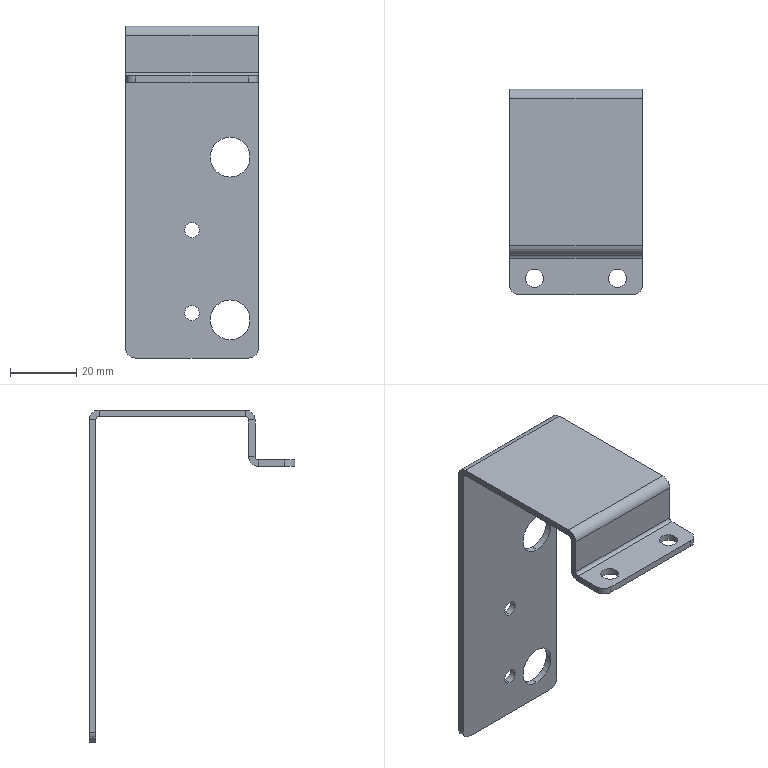Part | SolidWorks | features HoleWzd 3, Fillet 1, FlatPattern 1, SMBaseFlange 1, SheetMetal 1 | 1 solid | 46 faces | box 40 x 62 x 100 mm | volume 13167 mm3 | plane 24 | cylinder 22 | commonest cylinder face diameters 6 x7 4.5 x4 5.5 x4 12 x4 2 x3
STEP:
#1=CARTESIAN_POINT('',(31.5,50.,-94.5));
#2=VERTEX_POINT('',#1);
#3=CARTESIAN_POINT('',(31.5,50.,-82.5));
#4=VERTEX_POINT('',#3);
#5=CARTESIAN_POINT('',(31.5,50.,-88.5));
#6=DIRECTION('',(0.,1.,0.));
#7=DIRECTION('',(0.,0.,1.));
#8=AXIS2_PLACEMENT_3D('',#5,#6,#7);
#9=CIRCLE('',#8,6.);
#10=EDGE_CURVE('',#2,#4,#9,.T.);
#11=ORIENTED_EDGE('',*,*,#10,.T.);
#12=CARTESIAN_POINT('',(31.5,48.,-82.5));
#13=VERTEX_POINT('',#12);
#14=CARTESIAN_POINT('',(31.5,48.,-82.5));
#15=DIRECTION('',(0.,-1.,0.));
#16=VECTOR('',#15,1000.);
#17=LINE('',#14,#16);
#18=EDGE_CURVE('',#4,#13,#17,.T.);
#19=ORIENTED_EDGE('',*,*,#18,.T.);
#20=CARTESIAN_POINT('',(31.5,48.,-94.5));
#21=VERTEX_POINT('',#20);
#22=CARTESIAN_POINT('',(31.5,48.,-88.5));
#23=DIRECTION('',(0.,-1.,0.));
#24=DIRECTION('',(0.,0.,-1.));
#25=AXIS2_PLACEMENT_3D('',#22,#23,#24);
#26=CIRCLE('',#25,6.);
#27=EDGE_CURVE('',#13,#21,#26,.T.);
#28=ORIENTED_EDGE('',*,*,#27,.T.);
#29=CARTESIAN_POINT('',(31.5,48.,-94.5));
#30=DIRECTION('',(0.,-1.,0.));
#31=VECTOR('',#30,1000.);
#32=LINE('',#29,#31);
#33=EDGE_CURVE('',#2,#21,#32,.T.);
#34=ORIENTED_EDGE('',*,*,#33,.F.);
#35=EDGE_LOOP('',(#11,#19,#28,#34));
#36=FACE_OUTER_BOUND('',#35,.T.);
#37=CARTESIAN_POINT('',(31.5,48.,-88.5));
#38=DIRECTION('',(0.,-1.,0.));
#39=DIRECTION('',(0.,0.,-1.));
#40=AXIS2_PLACEMENT_3D('',#37,#38,#39);
#41=CYLINDRICAL_SURFACE('',#40,6.);
#42=ADVANCED_FACE('',(#36),#41,.F.);
#43=CARTESIAN_POINT('',(31.5,50.,-45.5));
#44=VERTEX_POINT('',#43);
#45=CARTESIAN_POINT('',(31.5,50.,-33.5));
#46=VERTEX_POINT('',#45);
#47=CARTESIAN_POINT('',(31.5,50.,-39.5));
#48=DIRECTION('',(0.,1.,0.));
#49=DIRECTION('',(0.,0.,1.));
#50=AXIS2_PLACEMENT_3D('',#47,#48,#49);
#51=CIRCLE('',#50,6.);
#52=EDGE_CURVE('',#44,#46,#51,.T.);
#53=ORIENTED_EDGE('',*,*,#52,.T.);
#54=CARTESIAN_POINT('',(31.5,48.,-33.5));
#55=VERTEX_POINT('',#54);
#56=CARTESIAN_POINT('',(31.5,48.,-33.5));
#57=DIRECTION('',(0.,-1.,0.));
#58=VECTOR('',#57,1000.);
#59=LINE('',#56,#58);
#60=EDGE_CURVE('',#46,#55,#59,.T.);
#61=ORIENTED_EDGE('',*,*,#60,.T.);
#62=CARTESIAN_POINT('',(31.5,48.,-45.5));
#63=VERTEX_POINT('',#62);
#64=CARTESIAN_POINT('',(31.5,48.,-39.5));
#65=DIRECTION('',(0.,-1.,0.));
#66=DIRECTION('',(0.,0.,-1.));
#67=AXIS2_PLACEMENT_3D('',#64,#65,#66);
#68=CIRCLE('',#67,6.);
#69=EDGE_CURVE('',#55,#63,#68,.T.);
#70=ORIENTED_EDGE('',*,*,#69,.T.);
#71=CARTESIAN_POINT('',(31.5,48.,-45.5));
#72=DIRECTION('',(0.,-1.,0.));
#73=VECTOR('',#72,1000.);
#74=LINE('',#71,#73);
#75=EDGE_CURVE('',#44,#63,#74,.T.);
#76=ORIENTED_EDGE('',*,*,#75,.F.);
#77=EDGE_LOOP('',(#53,#61,#70,#76));
#78=FACE_OUTER_BOUND('',#77,.T.);
#79=CARTESIAN_POINT('',(31.5,48.,-39.5));
#80=DIRECTION('',(0.,-1.,0.));
#81=DIRECTION('',(0.,0.,-1.));
#82=AXIS2_PLACEMENT_3D('',#79,#80,#81);
#83=CYLINDRICAL_SURFACE('',#82,6.);
#84=ADVANCED_FACE('',(#78),#83,.F.);
#85=CARTESIAN_POINT('',(20.,48.,-88.75));
#86=VERTEX_POINT('',#85);
#87=CARTESIAN_POINT('',(20.,48.,-84.25));
#88=VERTEX_POINT('',#87);
#89=CARTESIAN_POINT('',(20.,48.,-86.5));
#90=DIRECTION('',(0.,1.,0.));
#91=DIRECTION('',(0.,0.,1.));
#92=AXIS2_PLACEMENT_3D('',#89,#90,#91);
#93=CIRCLE('',#92,2.25);
#94=EDGE_CURVE('',#86,#88,#93,.T.);
#95=ORIENTED_EDGE('',*,*,#94,.F.);
#96=CARTESIAN_POINT('',(20.,50.,-88.75));
#97=VERTEX_POINT('',#96);
#98=CARTESIAN_POINT('',(20.,50.,-88.75));
#99=DIRECTION('',(0.,1.,0.));
#100=VECTOR('',#99,1000.);
#101=LINE('',#98,#100);
#102=EDGE_CURVE('',#86,#97,#101,.T.);
#103=ORIENTED_EDGE('',*,*,#102,.T.);
#104=CARTESIAN_POINT('',(20.,50.,-84.25));
#105=VERTEX_POINT('',#104);
#106=CARTESIAN_POINT('',(20.,50.,-86.5));
#107=DIRECTION('',(0.,1.,0.));
#108=DIRECTION('',(0.,0.,1.));
#109=AXIS2_PLACEMENT_3D('',#106,#107,#108);
#110=CIRCLE('',#109,2.25);
#111=EDGE_CURVE('',#97,#105,#110,.T.);
#112=ORIENTED_EDGE('',*,*,#111,.T.);
#113=CARTESIAN_POINT('',(20.,50.,-84.25));
#114=DIRECTION('',(0.,1.,0.));
#115=VECTOR('',#114,1000.);
#116=LINE('',#113,#115);
#117=EDGE_CURVE('',#88,#105,#116,.T.);
#118=ORIENTED_EDGE('',*,*,#117,.F.);
#119=EDGE_LOOP('',(#95,#103,#112,#118));
#120=FACE_OUTER_BOUND('',#119,.T.);
#121=CARTESIAN_POINT('',(20.,50.,-86.5));
#122=DIRECTION('',(0.,1.,0.));
#123=DIRECTION('',(0.,0.,1.));
#124=AXIS2_PLACEMENT_3D('',#121,#122,#123);
#125=CYLINDRICAL_SURFACE('',#124,2.25);
#126=ADVANCED_FACE('',(#120),#125,.F.);
#127=CARTESIAN_POINT('',(20.,48.,-63.75));
#128=VERTEX_POINT('',#127);
#129=CARTESIAN_POINT('',(20.,48.,-59.25));
#130=VERTEX_POINT('',#129);
#131=CARTESIAN_POINT('',(20.,48.,-61.5));
#132=DIRECTION('',(0.,1.,0.));
#133=DIRECTION('',(0.,0.,1.));
#134=AXIS2_PLACEMENT_3D('',#131,#132,#133);
#135=CIRCLE('',#134,2.25);
#136=EDGE_CURVE('',#128,#130,#135,.T.);
#137=ORIENTED_EDGE('',*,*,#136,.F.);
#138=CARTESIAN_POINT('',(20.,50.,-63.75));
#139=VERTEX_POINT('',#138);
#140=CARTESIAN_POINT('',(20.,50.,-63.75));
#141=DIRECTION('',(0.,1.,0.));
#142=VECTOR('',#141,1000.);
#143=LINE('',#140,#142);
#144=EDGE_CURVE('',#128,#139,#143,.T.);
#145=ORIENTED_EDGE('',*,*,#144,.T.);
#146=CARTESIAN_POINT('',(20.,50.,-59.25));
#147=VERTEX_POINT('',#146);
#148=CARTESIAN_POINT('',(20.,50.,-61.5));
#149=DIRECTION('',(0.,1.,0.));
#150=DIRECTION('',(0.,0.,1.));
#151=AXIS2_PLACEMENT_3D('',#148,#149,#150);
#152=CIRCLE('',#151,2.25);
#153=EDGE_CURVE('',#139,#147,#152,.T.);
#154=ORIENTED_EDGE('',*,*,#153,.T.);
#155=CARTESIAN_POINT('',(20.,50.,-59.25));
#156=DIRECTION('',(0.,1.,0.));
#157=VECTOR('',#156,1000.);
#158=LINE('',#155,#157);
#159=EDGE_CURVE('',#130,#147,#158,.T.);
#160=ORIENTED_EDGE('',*,*,#159,.F.);
#161=EDGE_LOOP('',(#137,#145,#154,#160));
#162=FACE_OUTER_BOUND('',#161,.T.);
#163=CARTESIAN_POINT('',(20.,50.,-61.5));
#164=DIRECTION('',(0.,1.,0.));
#165=DIRECTION('',(0.,0.,1.));
#166=AXIS2_PLACEMENT_3D('',#163,#164,#165);
#167=CYLINDRICAL_SURFACE('',#166,2.25);
#168=ADVANCED_FACE('',(#162),#167,.F.);
#169=CARTESIAN_POINT('',(4.75,-7.,-17.));
#170=VERTEX_POINT('',#169);
#171=CARTESIAN_POINT('',(10.25,-7.,-17.));
#172=VERTEX_POINT('',#171);
#173=CARTESIAN_POINT('',(7.5,-7.,-17.));
#174=DIRECTION('',(0.,0.,1.));
#175=DIRECTION('',(0.,-1.,0.));
#176=AXIS2_PLACEMENT_3D('',#173,#174,#175);
#177=CIRCLE('',#176,2.75);
#178=EDGE_CURVE('',#170,#172,#177,.T.);
#179=ORIENTED_EDGE('',*,*,#178,.F.);
#180=CARTESIAN_POINT('',(4.75,-7.,-15.));
#181=VERTEX_POINT('',#180);
#182=CARTESIAN_POINT('',(4.75,-7.,-15.));
#183=DIRECTION('',(0.,0.,1.));
#184=VECTOR('',#183,1000.);
#185=LINE('',#182,#184);
#186=EDGE_CURVE('',#170,#181,#185,.T.);
#187=ORIENTED_EDGE('',*,*,#186,.T.);
#188=CARTESIAN_POINT('',(10.25,-7.,-15.));
#189=VERTEX_POINT('',#188);
#190=CARTESIAN_POINT('',(7.5,-7.,-15.));
#191=DIRECTION('',(0.,0.,1.));
#192=DIRECTION('',(1.,0.,0.));
#193=AXIS2_PLACEMENT_3D('',#190,#191,#192);
#194=CIRCLE('',#193,2.75);
#195=EDGE_CURVE('',#181,#189,#194,.T.);
#196=ORIENTED_EDGE('',*,*,#195,.T.);
#197=CARTESIAN_POINT('',(10.25,-7.,-15.));
#198=DIRECTION('',(0.,0.,1.));
#199=VECTOR('',#198,1000.);
#200=LINE('',#197,#199);
#201=EDGE_CURVE('',#172,#189,#200,.T.);
#202=ORIENTED_EDGE('',*,*,#201,.F.);
#203=EDGE_LOOP('',(#179,#187,#196,#202));
#204=FACE_OUTER_BOUND('',#203,.T.);
#205=CARTESIAN_POINT('',(7.5,-7.,-15.));
#206=DIRECTION('',(0.,0.,1.));
#207=DIRECTION('',(1.,0.,0.));
#208=AXIS2_PLACEMENT_3D('',#205,#206,#207);
#209=CYLINDRICAL_SURFACE('',#208,2.75);
#210=ADVANCED_FACE('',(#204),#209,.F.);
#211=CARTESIAN_POINT('',(29.75,-7.,-17.));
#212=VERTEX_POINT('',#211);
#213=CARTESIAN_POINT('',(35.25,-7.,-17.));
#214=VERTEX_POINT('',#213);
#215=CARTESIAN_POINT('',(32.5,-7.,-17.));
#216=DIRECTION('',(0.,0.,1.));
#217=DIRECTION('',(0.,-1.,0.));
#218=AXIS2_PLACEMENT_3D('',#215,#216,#217);
#219=CIRCLE('',#218,2.75);
#220=EDGE_CURVE('',#212,#214,#219,.T.);
#221=ORIENTED_EDGE('',*,*,#220,.F.);
#222=CARTESIAN_POINT('',(29.75,-7.,-15.));
#223=VERTEX_POINT('',#222);
#224=CARTESIAN_POINT('',(29.75,-7.,-15.));
#225=DIRECTION('',(0.,0.,1.));
#226=VECTOR('',#225,1000.);
#227=LINE('',#224,#226);
#228=EDGE_CURVE('',#212,#223,#227,.T.);
#229=ORIENTED_EDGE('',*,*,#228,.T.);
#230=CARTESIAN_POINT('',(35.25,-7.,-15.));
#231=VERTEX_POINT('',#230);
#232=CARTESIAN_POINT('',(32.5,-7.,-15.));
#233=DIRECTION('',(0.,0.,1.));
#234=DIRECTION('',(1.,0.,0.));
#235=AXIS2_PLACEMENT_3D('',#232,#233,#234);
#236=CIRCLE('',#235,2.75);
#237=EDGE_CURVE('',#223,#231,#236,.T.);
#238=ORIENTED_EDGE('',*,*,#237,.T.);
#239=CARTESIAN_POINT('',(35.25,-7.,-15.));
#240=DIRECTION('',(0.,0.,1.));
#241=VECTOR('',#240,1000.);
#242=LINE('',#239,#241);
#243=EDGE_CURVE('',#214,#231,#242,.T.);
#244=ORIENTED_EDGE('',*,*,#243,.F.);
#245=EDGE_LOOP('',(#221,#229,#238,#244));
#246=FACE_OUTER_BOUND('',#245,.T.);
#247=CARTESIAN_POINT('',(32.5,-7.,-15.));
#248=DIRECTION('',(0.,0.,1.));
#249=DIRECTION('',(1.,0.,0.));
#250=AXIS2_PLACEMENT_3D('',#247,#248,#249);
#251=CYLINDRICAL_SURFACE('',#250,2.75);
#252=ADVANCED_FACE('',(#246),#251,.F.);
#253=CARTESIAN_POINT('',(40.,0.,-14.));
#254=VERTEX_POINT('',#253);
#255=CARTESIAN_POINT('',(40.,2.,-14.));
#256=VERTEX_POINT('',#255);
#257=CARTESIAN_POINT('',(40.,0.,-14.));
#258=DIRECTION('',(0.,1.,0.));
#259=VECTOR('',#258,1000.);
#260=LINE('',#257,#259);
#261=EDGE_CURVE('',#254,#256,#260,.T.);
#262=ORIENTED_EDGE('',*,*,#261,.F.);
#263=CARTESIAN_POINT('',(40.,-1.,-15.));
#264=VERTEX_POINT('',#263);
#265=CARTESIAN_POINT('',(40.,-1.,-14.));
#266=DIRECTION('',(1.,0.,0.));
#267=DIRECTION('',(0.,0.,1.));
#268=AXIS2_PLACEMENT_3D('',#265,#266,#267);
#269=CIRCLE('',#268,1.);
#270=EDGE_CURVE('',#264,#254,#269,.T.);
#271=ORIENTED_EDGE('',*,*,#270,.F.);
#272=CARTESIAN_POINT('',(40.,-1.,-17.));
#273=VERTEX_POINT('',#272);
#274=CARTESIAN_POINT('',(40.,-1.,-17.));
#275=DIRECTION('',(0.,0.,1.));
#276=VECTOR('',#275,1000.);
#277=LINE('',#274,#276);
#278=EDGE_CURVE('',#273,#264,#277,.T.);
#279=ORIENTED_EDGE('',*,*,#278,.F.);
#280=CARTESIAN_POINT('',(40.,-1.,-14.));
#281=DIRECTION('',(1.,0.,0.));
#282=DIRECTION('',(0.,0.,-1.));
#283=AXIS2_PLACEMENT_3D('',#280,#281,#282);
#284=CIRCLE('',#283,3.);
#285=EDGE_CURVE('',#273,#256,#284,.T.);
#286=ORIENTED_EDGE('',*,*,#285,.T.);
#287=EDGE_LOOP('',(#262,#271,#279,#286));
#288=FACE_OUTER_BOUND('',#287,.T.);
#289=CARTESIAN_POINT('',(40.,0.,-14.));
#290=DIRECTION('',(1.,0.,0.));
#291=DIRECTION('',(0.,0.,-1.));
#292=AXIS2_PLACEMENT_3D('',#289,#290,#291);
#293=PLANE('',#292);
#294=ADVANCED_FACE('',(#288),#293,.T.);
#295=CARTESIAN_POINT('',(40.,0.,-3.));
#296=VERTEX_POINT('',#295);
#297=CARTESIAN_POINT('',(40.,0.,0.));
#298=DIRECTION('',(0.,0.,1.));
#299=VECTOR('',#298,1000.);
#300=LINE('',#297,#299);
#301=EDGE_CURVE('',#254,#296,#300,.T.);
#302=ORIENTED_EDGE('',*,*,#301,.F.);
#303=ORIENTED_EDGE('',*,*,#261,.T.);
#304=CARTESIAN_POINT('',(40.,2.,-3.));
#305=VERTEX_POINT('',#304);
#306=CARTESIAN_POINT('',(40.,2.,0.));
#307=DIRECTION('',(0.,0.,1.));
#308=VECTOR('',#307,1000.);
#309=LINE('',#306,#308);
#310=EDGE_CURVE('',#256,#305,#309,.T.);
#311=ORIENTED_EDGE('',*,*,#310,.T.);
#312=CARTESIAN_POINT('',(40.,2.,-3.));
#313=DIRECTION('',(0.,-1.,0.));
#314=VECTOR('',#313,1000.);
#315=LINE('',#312,#314);
#316=EDGE_CURVE('',#305,#296,#315,.T.);
#317=ORIENTED_EDGE('',*,*,#316,.T.);
#318=EDGE_LOOP('',(#302,#303,#311,#317));
#319=FACE_OUTER_BOUND('',#318,.T.);
#320=CARTESIAN_POINT('',(40.,-1.,-17.));
#321=DIRECTION('',(1.,0.,0.));
#322=DIRECTION('',(0.,0.,-1.));
#323=AXIS2_PLACEMENT_3D('',#320,#321,#322);
#324=PLANE('',#323);
#325=ADVANCED_FACE('',(#319),#324,.T.);
#326=CARTESIAN_POINT('',(0.,-1.,-15.));
#327=VERTEX_POINT('',#326);
#328=CARTESIAN_POINT('',(0.,-1.,-17.));
#329=VERTEX_POINT('',#328);
#330=CARTESIAN_POINT('',(0.,-1.,-15.));
#331=DIRECTION('',(0.,0.,-1.));
#332=VECTOR('',#331,1000.);
#333=LINE('',#330,#332);
#334=EDGE_CURVE('',#327,#329,#333,.T.);
#335=ORIENTED_EDGE('',*,*,#334,.F.);
#336=CARTESIAN_POINT('',(0.,0.,-14.));
#337=VERTEX_POINT('',#336);
#338=CARTESIAN_POINT('',(0.,-1.,-14.));
#339=DIRECTION('',(1.,0.,0.));
#340=DIRECTION('',(0.,0.,1.));
#341=AXIS2_PLACEMENT_3D('',#338,#339,#340);
#342=CIRCLE('',#341,1.);
#343=EDGE_CURVE('',#327,#337,#342,.T.);
#344=ORIENTED_EDGE('',*,*,#343,.T.);
#345=CARTESIAN_POINT('',(0.,2.,-14.));
#346=VERTEX_POINT('',#345);
#347=CARTESIAN_POINT('',(0.,2.,-14.));
#348=DIRECTION('',(0.,-1.,0.));
#349=VECTOR('',#348,1000.);
#350=LINE('',#347,#349);
#351=EDGE_CURVE('',#346,#337,#350,.T.);
#352=ORIENTED_EDGE('',*,*,#351,.F.);
#353=CARTESIAN_POINT('',(0.,-1.,-14.));
#354=DIRECTION('',(1.,0.,0.));
#355=DIRECTION('',(0.,0.,-1.));
#356=AXIS2_PLACEMENT_3D('',#353,#354,#355);
#357=CIRCLE('',#356,3.);
#358=EDGE_CURVE('',#329,#346,#357,.T.);
#359=ORIENTED_EDGE('',*,*,#358,.F.);
#360=EDGE_LOOP('',(#335,#344,#352,#359));
#361=FACE_OUTER_BOUND('',#360,.T.);
#362=CARTESIAN_POINT('',(0.,-1.,-15.));
#363=DIRECTION('',(-1.,0.,0.));
#364=DIRECTION('',(0.,0.,1.));
#365=AXIS2_PLACEMENT_3D('',#362,#363,#364);
#366=PLANE('',#365);
#367=ADVANCED_FACE('',(#361),#366,.T.);
#368=CARTESIAN_POINT('',(0.,-9.,-17.));
#369=VERTEX_POINT('',#368);
#370=CARTESIAN_POINT('',(0.,0.,-17.));
#371=DIRECTION('',(0.,1.,0.));
#372=VECTOR('',#371,1000.);
#373=LINE('',#370,#372);
#374=EDGE_CURVE('',#369,#329,#373,.T.);
#375=ORIENTED_EDGE('',*,*,#374,.F.);
#376=CARTESIAN_POINT('',(0.,-9.,-15.));
#377=VERTEX_POINT('',#376);
#378=CARTESIAN_POINT('',(0.,-9.,-14.));
#379=DIRECTION('',(0.,0.,1.));
#380=VECTOR('',#379,1000.);
#381=LINE('',#378,#380);
#382=EDGE_CURVE('',#369,#377,#381,.T.);
#383=ORIENTED_EDGE('',*,*,#382,.T.);
#384=CARTESIAN_POINT('',(0.,0.,-15.));
#385=DIRECTION('',(0.,1.,0.));
#386=VECTOR('',#385,1000.);
#387=LINE('',#384,#386);
#388=EDGE_CURVE('',#377,#327,#387,.T.);
#389=ORIENTED_EDGE('',*,*,#388,.T.);
#390=ORIENTED_EDGE('',*,*,#334,.T.);
#391=EDGE_LOOP('',(#375,#383,#389,#390));
#392=FACE_OUTER_BOUND('',#391,.T.);
#393=CARTESIAN_POINT('',(0.,2.,-14.));
#394=DIRECTION('',(-1.,0.,0.));
#395=DIRECTION('',(0.,0.,1.));
#396=AXIS2_PLACEMENT_3D('',#393,#394,#395);
#397=PLANE('',#396);
#398=ADVANCED_FACE('',(#392),#397,.T.);
#399=CARTESIAN_POINT('',(40.,3.,0.));
#400=VERTEX_POINT('',#399);
#401=CARTESIAN_POINT('',(40.,3.,-2.));
#402=VERTEX_POINT('',#401);
#403=CARTESIAN_POINT('',(40.,3.,0.));
#404=DIRECTION('',(0.,0.,-1.));
#405=VECTOR('',#404,1000.);
#406=LINE('',#403,#405);
#407=EDGE_CURVE('',#400,#402,#406,.T.);
#408=ORIENTED_EDGE('',*,*,#407,.F.);
#409=CARTESIAN_POINT('',(40.,3.,-3.));
#410=DIRECTION('',(-1.,0.,0.));
#411=DIRECTION('',(0.,0.,-1.));
#412=AXIS2_PLACEMENT_3D('',#409,#410,#411);
#413=CIRCLE('',#412,3.);
#414=EDGE_CURVE('',#296,#400,#413,.T.);
#415=ORIENTED_EDGE('',*,*,#414,.F.);
#416=ORIENTED_EDGE('',*,*,#316,.F.);
#417=CARTESIAN_POINT('',(40.,3.,-3.));
#418=DIRECTION('',(-1.,0.,0.));
#419=DIRECTION('',(0.,0.,-1.));
#420=AXIS2_PLACEMENT_3D('',#417,#418,#419);
#421=CIRCLE('',#420,1.);
#422=EDGE_CURVE('',#305,#402,#421,.T.);
#423=ORIENTED_EDGE('',*,*,#422,.T.);
#424=EDGE_LOOP('',(#408,#415,#416,#423));
#425=FACE_OUTER_BOUND('',#424,.T.);
#426=CARTESIAN_POINT('',(40.,3.,0.));
#427=DIRECTION('',(1.,0.,0.));
#428=DIRECTION('',(0.,0.,-1.));
#429=AXIS2_PLACEMENT_3D('',#426,#427,#428);
#430=PLANE('',#429);
#431=ADVANCED_FACE('',(#425),#430,.T.);
#432=CARTESIAN_POINT('',(40.,47.,0.));
#433=VERTEX_POINT('',#432);
#434=CARTESIAN_POINT('',(40.,0.,0.));
#435=DIRECTION('',(0.,1.,0.));
#436=VECTOR('',#435,1000.);
#437=LINE('',#434,#436);
#438=EDGE_CURVE('',#400,#433,#437,.T.);
#439=ORIENTED_EDGE('',*,*,#438,.F.);
#440=ORIENTED_EDGE('',*,*,#407,.T.);
#441=CARTESIAN_POINT('',(40.,47.,-2.));
#442=VERTEX_POINT('',#441);
#443=CARTESIAN_POINT('',(40.,0.,-2.));
#444=DIRECTION('',(0.,1.,0.));
#445=VECTOR('',#444,1000.);
#446=LINE('',#443,#445);
#447=EDGE_CURVE('',#402,#442,#446,.T.);
#448=ORIENTED_EDGE('',*,*,#447,.T.);
#449=CARTESIAN_POINT('',(40.,47.,-2.));
#450=DIRECTION('',(0.,0.,1.));
#451=VECTOR('',#450,1000.);
#452=LINE('',#449,#451);
#453=EDGE_CURVE('',#442,#433,#452,.T.);
#454=ORIENTED_EDGE('',*,*,#453,.T.);
#455=EDGE_LOOP('',(#439,#440,#448,#454));
#456=FACE_OUTER_BOUND('',#455,.T.);
#457=CARTESIAN_POINT('',(40.,2.,-3.));
#458=DIRECTION('',(1.,0.,0.));
#459=DIRECTION('',(0.,0.,-1.));
#460=AXIS2_PLACEMENT_3D('',#457,#458,#459);
#461=PLANE('',#460);
#462=ADVANCED_FACE('',(#456),#461,.T.);
#463=CARTESIAN_POINT('',(0.,0.,-3.));
#464=VERTEX_POINT('',#463);
#465=CARTESIAN_POINT('',(0.,2.,-3.));
#466=VERTEX_POINT('',#465);
#467=CARTESIAN_POINT('',(0.,0.,-3.));
#468=DIRECTION('',(0.,1.,0.));
#469=VECTOR('',#468,1000.);
#470=LINE('',#467,#469);
#471=EDGE_CURVE('',#464,#466,#470,.T.);
#472=ORIENTED_EDGE('',*,*,#471,.F.);
#473=CARTESIAN_POINT('',(0.,3.,0.));
#474=VERTEX_POINT('',#473);
#475=CARTESIAN_POINT('',(0.,3.,-3.));
#476=DIRECTION('',(-1.,0.,0.));
#477=DIRECTION('',(0.,0.,-1.));
#478=AXIS2_PLACEMENT_3D('',#475,#476,#477);
#479=CIRCLE('',#478,3.);
#480=EDGE_CURVE('',#464,#474,#479,.T.);
#481=ORIENTED_EDGE('',*,*,#480,.T.);
#482=CARTESIAN_POINT('',(0.,3.,-2.));
#483=VERTEX_POINT('',#482);
#484=CARTESIAN_POINT('',(0.,3.,-2.));
#485=DIRECTION('',(0.,0.,1.));
#486=VECTOR('',#485,1000.);
#487=LINE('',#484,#486);
#488=EDGE_CURVE('',#483,#474,#487,.T.);
#489=ORIENTED_EDGE('',*,*,#488,.F.);
#490=CARTESIAN_POINT('',(0.,3.,-3.));
#491=DIRECTION('',(-1.,0.,0.));
#492=DIRECTION('',(0.,0.,-1.));
#493=AXIS2_PLACEMENT_3D('',#490,#491,#492);
#494=CIRCLE('',#493,1.);
#495=EDGE_CURVE('',#466,#483,#494,.T.);
#496=ORIENTED_EDGE('',*,*,#495,.F.);
#497=EDGE_LOOP('',(#472,#481,#489,#496));
#498=FACE_OUTER_BOUND('',#497,.T.);
#499=CARTESIAN_POINT('',(0.,0.,-3.));
#500=DIRECTION('',(-1.,0.,0.));
#501=DIRECTION('',(0.,0.,1.));
#502=AXIS2_PLACEMENT_3D('',#499,#500,#501);
#503=PLANE('',#502);
#504=ADVANCED_FACE('',(#498),#503,.T.);
#505=CARTESIAN_POINT('',(0.,0.,0.));
#506=DIRECTION('',(0.,0.,1.));
#507=VECTOR('',#506,1000.);
#508=LINE('',#505,#507);
#509=EDGE_CURVE('',#337,#464,#508,.T.);
#510=ORIENTED_EDGE('',*,*,#509,.T.);
#511=ORIENTED_EDGE('',*,*,#471,.T.);
#512=CARTESIAN_POINT('',(0.,2.,0.));
#513=DIRECTION('',(0.,0.,1.));
#514=VECTOR('',#513,1000.);
#515=LINE('',#512,#514);
#516=EDGE_CURVE('',#346,#466,#515,.T.);
#517=ORIENTED_EDGE('',*,*,#516,.F.);
#518=ORIENTED_EDGE('',*,*,#351,.T.);
#519=EDGE_LOOP('',(#510,#511,#517,#518));
#520=FACE_OUTER_BOUND('',#519,.T.);
#521=CARTESIAN_POINT('',(0.,3.,-2.));
#522=DIRECTION('',(-1.,0.,0.));
#523=DIRECTION('',(0.,0.,1.));
#524=AXIS2_PLACEMENT_3D('',#521,#522,#523);
#525=PLANE('',#524);
#526=ADVANCED_FACE('',(#520),#525,.T.);
#527=CARTESIAN_POINT('',(40.,50.,-3.));
#528=VERTEX_POINT('',#527);
#529=CARTESIAN_POINT('',(40.,48.,-3.));
#530=VERTEX_POINT('',#529);
#531=CARTESIAN_POINT('',(40.,50.,-3.));
#532=DIRECTION('',(0.,-1.,0.));
#533=VECTOR('',#532,1000.);
#534=LINE('',#531,#533);
#535=EDGE_CURVE('',#528,#530,#534,.T.);
#536=ORIENTED_EDGE('',*,*,#535,.F.);
#537=CARTESIAN_POINT('',(40.,47.,-3.));
#538=DIRECTION('',(-1.,0.,0.));
#539=DIRECTION('',(0.,0.,-1.));
#540=AXIS2_PLACEMENT_3D('',#537,#538,#539);
#541=CIRCLE('',#540,3.);
#542=EDGE_CURVE('',#433,#528,#541,.T.);
#543=ORIENTED_EDGE('',*,*,#542,.F.);
#544=ORIENTED_EDGE('',*,*,#453,.F.);
#545=CARTESIAN_POINT('',(40.,47.,-3.));
#546=DIRECTION('',(-1.,0.,0.));
#547=DIRECTION('',(0.,0.,-1.));
#548=AXIS2_PLACEMENT_3D('',#545,#546,#547);
#549=CIRCLE('',#548,1.);
#550=EDGE_CURVE('',#442,#530,#549,.T.);
#551=ORIENTED_EDGE('',*,*,#550,.T.);
#552=EDGE_LOOP('',(#536,#543,#544,#551));
#553=FACE_OUTER_BOUND('',#552,.T.);
#554=CARTESIAN_POINT('',(40.,50.,-3.));
#555=DIRECTION('',(1.,0.,0.));
#556=DIRECTION('',(0.,0.,-1.));
#557=AXIS2_PLACEMENT_3D('',#554,#555,#556);
#558=PLANE('',#557);
#559=ADVANCED_FACE('',(#553),#558,.T.);
#560=CARTESIAN_POINT('',(40.,48.,-97.));
#561=VERTEX_POINT('',#560);
#562=CARTESIAN_POINT('',(40.,48.,0.));
#563=DIRECTION('',(0.,0.,-1.));
#564=VECTOR('',#563,1000.);
#565=LINE('',#562,#564);
#566=EDGE_CURVE('',#530,#561,#565,.T.);
#567=ORIENTED_EDGE('',*,*,#566,.T.);
#568=CARTESIAN_POINT('',(40.,50.,-97.));
#569=VERTEX_POINT('',#568);
#570=CARTESIAN_POINT('',(40.,47.,-97.));
#571=DIRECTION('',(0.,1.,0.));
#572=VECTOR('',#571,1000.);
#573=LINE('',#570,#572);
#574=EDGE_CURVE('',#561,#569,#573,.T.);
#575=ORIENTED_EDGE('',*,*,#574,.T.);
#576=CARTESIAN_POINT('',(40.,50.,0.));
#577=DIRECTION('',(0.,0.,-1.));
#578=VECTOR('',#577,1000.);
#579=LINE('',#576,#578);
#580=EDGE_CURVE('',#528,#569,#579,.T.);
#581=ORIENTED_EDGE('',*,*,#580,.F.);
#582=ORIENTED_EDGE('',*,*,#535,.T.);
#583=EDGE_LOOP('',(#567,#575,#581,#582));
#584=FACE_OUTER_BOUND('',#583,.T.);
#585=CARTESIAN_POINT('',(40.,47.,-2.));
#586=DIRECTION('',(1.,0.,0.));
#587=DIRECTION('',(0.,0.,-1.));
#588=AXIS2_PLACEMENT_3D('',#585,#586,#587);
#589=PLANE('',#588);
#590=ADVANCED_FACE('',(#584),#589,.T.);
#591=CARTESIAN_POINT('',(0.,47.,0.));
#592=VERTEX_POINT('',#591);
#593=CARTESIAN_POINT('',(0.,47.,-2.));
#594=VERTEX_POINT('',#593);
#595=CARTESIAN_POINT('',(0.,47.,0.));
#596=DIRECTION('',(0.,0.,-1.));
#597=VECTOR('',#596,1000.);
#598=LINE('',#595,#597);
#599=EDGE_CURVE('',#592,#594,#598,.T.);
#600=ORIENTED_EDGE('',*,*,#599,.F.);
#601=CARTESIAN_POINT('',(0.,50.,-3.));
#602=VERTEX_POINT('',#601);
#603=CARTESIAN_POINT('',(0.,47.,-3.));
#604=DIRECTION('',(-1.,0.,0.));
#605=DIRECTION('',(0.,0.,-1.));
#606=AXIS2_PLACEMENT_3D('',#603,#604,#605);
#607=CIRCLE('',#606,3.);
#608=EDGE_CURVE('',#592,#602,#607,.T.);
#609=ORIENTED_EDGE('',*,*,#608,.T.);
#610=CARTESIAN_POINT('',(0.,48.,-3.));
#611=VERTEX_POINT('',#610);
#612=CARTESIAN_POINT('',(0.,48.,-3.));
#613=DIRECTION('',(0.,1.,0.));
#614=VECTOR('',#613,1000.);
#615=LINE('',#612,#614);
#616=EDGE_CURVE('',#611,#602,#615,.T.);
#617=ORIENTED_EDGE('',*,*,#616,.F.);
#618=CARTESIAN_POINT('',(0.,47.,-3.));
#619=DIRECTION('',(-1.,0.,0.));
#620=DIRECTION('',(0.,0.,-1.));
#621=AXIS2_PLACEMENT_3D('',#618,#619,#620);
#622=CIRCLE('',#621,1.);
#623=EDGE_CURVE('',#594,#611,#622,.T.);
#624=ORIENTED_EDGE('',*,*,#623,.F.);
#625=EDGE_LOOP('',(#600,#609,#617,#624));
#626=FACE_OUTER_BOUND('',#625,.T.);
#627=CARTESIAN_POINT('',(0.,47.,0.));
#628=DIRECTION('',(-1.,0.,0.));
#629=DIRECTION('',(0.,0.,1.));
#630=AXIS2_PLACEMENT_3D('',#627,#628,#629);
#631=PLANE('',#630);
#632=ADVANCED_FACE('',(#626),#631,.T.);
#633=CARTESIAN_POINT('',(0.,0.,0.));
#634=DIRECTION('',(0.,1.,0.));
#635=VECTOR('',#634,1000.);
#636=LINE('',#633,#635);
#637=EDGE_CURVE('',#474,#592,#636,.T.);
#638=ORIENTED_EDGE('',*,*,#637,.T.);
#639=ORIENTED_EDGE('',*,*,#599,.T.);
#640=CARTESIAN_POINT('',(0.,0.,-2.));
#641=DIRECTION('',(0.,1.,0.));
#642=VECTOR('',#641,1000.);
#643=LINE('',#640,#642);
#644=EDGE_CURVE('',#483,#594,#643,.T.);
#645=ORIENTED_EDGE('',*,*,#644,.F.);
#646=ORIENTED_EDGE('',*,*,#488,.T.);
#647=EDGE_LOOP('',(#638,#639,#645,#646));
#648=FACE_OUTER_BOUND('',#647,.T.);
#649=CARTESIAN_POINT('',(0.,48.,-3.));
#650=DIRECTION('',(-1.,0.,0.));
#651=DIRECTION('',(0.,0.,1.));
#652=AXIS2_PLACEMENT_3D('',#649,#650,#651);
#653=PLANE('',#652);
#654=ADVANCED_FACE('',(#648),#653,.T.);
#655=CARTESIAN_POINT('',(31.5,48.,-88.5));
#656=DIRECTION('',(0.,-1.,0.));
#657=DIRECTION('',(0.,0.,-1.));
#658=AXIS2_PLACEMENT_3D('',#655,#656,#657);
#659=CIRCLE('',#658,6.);
#660=EDGE_CURVE('',#21,#13,#659,.T.);
#661=ORIENTED_EDGE('',*,*,#660,.F.);
#662=ORIENTED_EDGE('',*,*,#27,.F.);
#663=EDGE_LOOP('',(#661,#662));
#664=FACE_BOUND('',#663,.T.);
#665=CARTESIAN_POINT('',(31.5,48.,-39.5));
#666=DIRECTION('',(0.,-1.,0.));
#667=DIRECTION('',(0.,0.,-1.));
#668=AXIS2_PLACEMENT_3D('',#665,#666,#667);
#669=CIRCLE('',#668,6.);
#670=EDGE_CURVE('',#63,#55,#669,.T.);
#671=ORIENTED_EDGE('',*,*,#670,.F.);
#672=ORIENTED_EDGE('',*,*,#69,.F.);
#673=EDGE_LOOP('',(#671,#672));
#674=FACE_BOUND('',#673,.T.);
#675=CARTESIAN_POINT('',(20.,48.,-86.5));
#676=DIRECTION('',(0.,1.,0.));
#677=DIRECTION('',(0.,0.,1.));
#678=AXIS2_PLACEMENT_3D('',#675,#676,#677);
#679=CIRCLE('',#678,2.25);
#680=EDGE_CURVE('',#88,#86,#679,.T.);
#681=ORIENTED_EDGE('',*,*,#680,.T.);
#682=ORIENTED_EDGE('',*,*,#94,.T.);
#683=EDGE_LOOP('',(#681,#682));
#684=FACE_BOUND('',#683,.T.);
#685=CARTESIAN_POINT('',(20.,48.,-61.5));
#686=DIRECTION('',(0.,1.,0.));
#687=DIRECTION('',(0.,0.,1.));
#688=AXIS2_PLACEMENT_3D('',#685,#686,#687);
#689=CIRCLE('',#688,2.25);
#690=EDGE_CURVE('',#130,#128,#689,.T.);
#691=ORIENTED_EDGE('',*,*,#690,.T.);
#692=ORIENTED_EDGE('',*,*,#136,.T.);
#693=EDGE_LOOP('',(#691,#692));
#694=FACE_BOUND('',#693,.T.);
#695=CARTESIAN_POINT('',(37.,48.,-100.));
#696=VERTEX_POINT('',#695);
#697=CARTESIAN_POINT('',(3.,48.,-100.));
#698=VERTEX_POINT('',#697);
#699=CARTESIAN_POINT('',(40.,48.,-100.));
#700=DIRECTION('',(-1.,0.,0.));
#701=VECTOR('',#700,1000.);
#702=LINE('',#699,#701);
#703=EDGE_CURVE('',#696,#698,#702,.T.);
#704=ORIENTED_EDGE('',*,*,#703,.F.);
#705=CARTESIAN_POINT('',(37.,48.,-97.));
#706=DIRECTION('',(0.,-1.,0.));
#707=DIRECTION('',(0.,0.,1.));
#708=AXIS2_PLACEMENT_3D('',#705,#706,#707);
#709=CIRCLE('',#708,3.);
#710=EDGE_CURVE('',#696,#561,#709,.T.);
#711=ORIENTED_EDGE('',*,*,#710,.T.);
#712=ORIENTED_EDGE('',*,*,#566,.F.);
#713=CARTESIAN_POINT('',(40.,48.,-3.));
#714=DIRECTION('',(-1.,0.,0.));
#715=VECTOR('',#714,1000.);
#716=LINE('',#713,#715);
#717=EDGE_CURVE('',#530,#611,#716,.T.);
#718=ORIENTED_EDGE('',*,*,#717,.T.);
#719=CARTESIAN_POINT('',(0.,48.,-97.));
#720=VERTEX_POINT('',#719);
#721=CARTESIAN_POINT('',(0.,48.,0.));
#722=DIRECTION('',(0.,0.,-1.));
#723=VECTOR('',#722,1000.);
#724=LINE('',#721,#723);
#725=EDGE_CURVE('',#611,#720,#724,.T.);
#726=ORIENTED_EDGE('',*,*,#725,.T.);
#727=CARTESIAN_POINT('',(3.,48.,-97.));
#728=DIRECTION('',(0.,-1.,0.));
#729=DIRECTION('',(0.,0.,1.));
#730=AXIS2_PLACEMENT_3D('',#727,#728,#729);
#731=CIRCLE('',#730,3.);
#732=EDGE_CURVE('',#720,#698,#731,.T.);
#733=ORIENTED_EDGE('',*,*,#732,.T.);
#734=EDGE_LOOP('',(#704,#711,#712,#718,#726,#733));
#735=FACE_OUTER_BOUND('',#734,.T.);
#736=CARTESIAN_POINT('',(40.,48.,0.));
#737=DIRECTION('',(0.,1.,0.));
#738=DIRECTION('',(0.,0.,1.));
#739=AXIS2_PLACEMENT_3D('',#736,#737,#738);
#740=PLANE('',#739);
#741=ADVANCED_FACE('',(#664,#674,#684,#694,#735),#740,.F.);
#742=CARTESIAN_POINT('',(37.,50.,-100.));
#743=VERTEX_POINT('',#742);
#744=CARTESIAN_POINT('',(3.,50.,-100.));
#745=VERTEX_POINT('',#744);
#746=CARTESIAN_POINT('',(40.,50.,-100.));
#747=DIRECTION('',(-1.,0.,0.));
#748=VECTOR('',#747,1000.);
#749=LINE('',#746,#748);
#750=EDGE_CURVE('',#743,#745,#749,.T.);
#751=ORIENTED_EDGE('',*,*,#750,.F.);
#752=CARTESIAN_POINT('',(37.,50.,-100.));
#753=DIRECTION('',(0.,-1.,0.));
#754=VECTOR('',#753,1000.);
#755=LINE('',#752,#754);
#756=EDGE_CURVE('',#743,#696,#755,.T.);
#757=ORIENTED_EDGE('',*,*,#756,.T.);
#758=ORIENTED_EDGE('',*,*,#703,.T.);
#759=CARTESIAN_POINT('',(3.,50.,-100.));
#760=DIRECTION('',(0.,1.,0.));
#761=VECTOR('',#760,1000.);
#762=LINE('',#759,#761);
#763=EDGE_CURVE('',#698,#745,#762,.T.);
#764=ORIENTED_EDGE('',*,*,#763,.T.);
#765=EDGE_LOOP('',(#751,#757,#758,#764));
#766=FACE_OUTER_BOUND('',#765,.T.);
#767=CARTESIAN_POINT('',(40.,50.,-100.));
#768=DIRECTION('',(0.,0.,-1.));
#769=DIRECTION('',(-1.,0.,0.));
#770=AXIS2_PLACEMENT_3D('',#767,#768,#769);
#771=PLANE('',#770);
#772=ADVANCED_FACE('',(#766),#771,.T.);
#773=ORIENTED_EDGE('',*,*,#10,.F.);
#774=CARTESIAN_POINT('',(31.5,50.,-88.5));
#775=DIRECTION('',(0.,1.,0.));
#776=DIRECTION('',(0.,0.,1.));
#777=AXIS2_PLACEMENT_3D('',#774,#775,#776);
#778=CIRCLE('',#777,6.);
#779=EDGE_CURVE('',#4,#2,#778,.T.);
#780=ORIENTED_EDGE('',*,*,#779,.F.);
#781=EDGE_LOOP('',(#773,#780));
#782=FACE_BOUND('',#781,.T.);
#783=ORIENTED_EDGE('',*,*,#52,.F.);
#784=CARTESIAN_POINT('',(31.5,50.,-39.5));
#785=DIRECTION('',(0.,1.,0.));
#786=DIRECTION('',(0.,0.,1.));
#787=AXIS2_PLACEMENT_3D('',#784,#785,#786);
#788=CIRCLE('',#787,6.);
#789=EDGE_CURVE('',#46,#44,#788,.T.);
#790=ORIENTED_EDGE('',*,*,#789,.F.);
#791=EDGE_LOOP('',(#783,#790));
#792=FACE_BOUND('',#791,.T.);
#793=CARTESIAN_POINT('',(20.,50.,-86.5));
#794=DIRECTION('',(0.,1.,0.));
#795=DIRECTION('',(0.,0.,1.));
#796=AXIS2_PLACEMENT_3D('',#793,#794,#795);
#797=CIRCLE('',#796,2.25);
#798=EDGE_CURVE('',#105,#97,#797,.T.);
#799=ORIENTED_EDGE('',*,*,#798,.F.);
#800=ORIENTED_EDGE('',*,*,#111,.F.);
#801=EDGE_LOOP('',(#799,#800));
#802=FACE_BOUND('',#801,.T.);
#803=CARTESIAN_POINT('',(20.,50.,-61.5));
#804=DIRECTION('',(0.,1.,0.));
#805=DIRECTION('',(0.,0.,1.));
#806=AXIS2_PLACEMENT_3D('',#803,#804,#805);
#807=CIRCLE('',#806,2.25);
#808=EDGE_CURVE('',#147,#139,#807,.T.);
#809=ORIENTED_EDGE('',*,*,#808,.F.);
#810=ORIENTED_EDGE('',*,*,#153,.F.);
#811=EDGE_LOOP('',(#809,#810));
#812=FACE_BOUND('',#811,.T.);
#813=ORIENTED_EDGE('',*,*,#580,.T.);
#814=CARTESIAN_POINT('',(37.,50.,-97.));
#815=DIRECTION('',(0.,1.,0.));
#816=DIRECTION('',(0.,0.,1.));
#817=AXIS2_PLACEMENT_3D('',#814,#815,#816);
#818=CIRCLE('',#817,3.);
#819=EDGE_CURVE('',#569,#743,#818,.T.);
#820=ORIENTED_EDGE('',*,*,#819,.T.);
#821=ORIENTED_EDGE('',*,*,#750,.T.);
#822=CARTESIAN_POINT('',(0.,50.,-97.));
#823=VERTEX_POINT('',#822);
#824=CARTESIAN_POINT('',(3.,50.,-97.));
#825=DIRECTION('',(0.,1.,0.));
#826=DIRECTION('',(0.,0.,1.));
#827=AXIS2_PLACEMENT_3D('',#824,#825,#826);
#828=CIRCLE('',#827,3.);
#829=EDGE_CURVE('',#745,#823,#828,.T.);
#830=ORIENTED_EDGE('',*,*,#829,.T.);
#831=CARTESIAN_POINT('',(0.,50.,0.));
#832=DIRECTION('',(0.,0.,-1.));
#833=VECTOR('',#832,1000.);
#834=LINE('',#831,#833);
#835=EDGE_CURVE('',#602,#823,#834,.T.);
#836=ORIENTED_EDGE('',*,*,#835,.F.);
#837=CARTESIAN_POINT('',(40.,50.,-3.));
#838=DIRECTION('',(-1.,0.,0.));
#839=VECTOR('',#838,1000.);
#840=LINE('',#837,#839);
#841=EDGE_CURVE('',#528,#602,#840,.T.);
#842=ORIENTED_EDGE('',*,*,#841,.F.);
#843=EDGE_LOOP('',(#813,#820,#821,#830,#836,#842));
#844=FACE_OUTER_BOUND('',#843,.T.);
#845=CARTESIAN_POINT('',(40.,50.,0.));
#846=DIRECTION('',(0.,1.,0.));
#847=DIRECTION('',(0.,0.,1.));
#848=AXIS2_PLACEMENT_3D('',#845,#846,#847);
#849=PLANE('',#848);
#850=ADVANCED_FACE('',(#782,#792,#802,#812,#844),#849,.T.);
#851=ORIENTED_EDGE('',*,*,#608,.F.);
#852=CARTESIAN_POINT('',(40.,47.,0.));
#853=DIRECTION('',(-1.,0.,0.));
#854=VECTOR('',#853,1000.);
#855=LINE('',#852,#854);
#856=EDGE_CURVE('',#433,#592,#855,.T.);
#857=ORIENTED_EDGE('',*,*,#856,.F.);
#858=ORIENTED_EDGE('',*,*,#542,.T.);
#859=ORIENTED_EDGE('',*,*,#841,.T.);
#860=EDGE_LOOP('',(#851,#857,#858,#859));
#861=FACE_OUTER_BOUND('',#860,.T.);
#862=CARTESIAN_POINT('',(40.,47.,-3.));
#863=DIRECTION('',(-1.,0.,0.));
#864=DIRECTION('',(0.,0.,1.));
#865=AXIS2_PLACEMENT_3D('',#862,#863,#864);
#866=CYLINDRICAL_SURFACE('',#865,3.);
#867=ADVANCED_FACE('',(#861),#866,.T.);
#868=ORIENTED_EDGE('',*,*,#637,.F.);
#869=CARTESIAN_POINT('',(40.,3.,0.));
#870=DIRECTION('',(-1.,0.,0.));
#871=VECTOR('',#870,1000.);
#872=LINE('',#869,#871);
#873=EDGE_CURVE('',#400,#474,#872,.T.);
#874=ORIENTED_EDGE('',*,*,#873,.F.);
#875=ORIENTED_EDGE('',*,*,#438,.T.);
#876=ORIENTED_EDGE('',*,*,#856,.T.);
#877=EDGE_LOOP('',(#868,#874,#875,#876));
#878=FACE_OUTER_BOUND('',#877,.T.);
#879=CARTESIAN_POINT('',(40.,0.,0.));
#880=DIRECTION('',(0.,0.,1.));
#881=DIRECTION('',(1.,0.,0.));
#882=AXIS2_PLACEMENT_3D('',#879,#880,#881);
#883=PLANE('',#882);
#884=ADVANCED_FACE('',(#878),#883,.T.);
#885=ORIENTED_EDGE('',*,*,#480,.F.);
#886=CARTESIAN_POINT('',(40.,0.,-3.));
#887=DIRECTION('',(-1.,0.,0.));
#888=VECTOR('',#887,1000.);
#889=LINE('',#886,#888);
#890=EDGE_CURVE('',#296,#464,#889,.T.);
#891=ORIENTED_EDGE('',*,*,#890,.F.);
#892=ORIENTED_EDGE('',*,*,#414,.T.);
#893=ORIENTED_EDGE('',*,*,#873,.T.);
#894=EDGE_LOOP('',(#885,#891,#892,#893));
#895=FACE_OUTER_BOUND('',#894,.T.);
#896=CARTESIAN_POINT('',(40.,3.,-3.));
#897=DIRECTION('',(-1.,0.,0.));
#898=DIRECTION('',(0.,0.,1.));
#899=AXIS2_PLACEMENT_3D('',#896,#897,#898);
#900=CYLINDRICAL_SURFACE('',#899,3.);
#901=ADVANCED_FACE('',(#895),#900,.T.);
#902=ORIENTED_EDGE('',*,*,#509,.F.);
#903=CARTESIAN_POINT('',(40.,0.,-14.));
#904=DIRECTION('',(-1.,0.,0.));
#905=VECTOR('',#904,1000.);
#906=LINE('',#903,#905);
#907=EDGE_CURVE('',#254,#337,#906,.T.);
#908=ORIENTED_EDGE('',*,*,#907,.F.);
#909=ORIENTED_EDGE('',*,*,#301,.T.);
#910=ORIENTED_EDGE('',*,*,#890,.T.);
#911=EDGE_LOOP('',(#902,#908,#909,#910));
#912=FACE_OUTER_BOUND('',#911,.T.);
#913=CARTESIAN_POINT('',(40.,0.,0.));
#914=DIRECTION('',(0.,-1.,0.));
#915=DIRECTION('',(0.,0.,-1.));
#916=AXIS2_PLACEMENT_3D('',#913,#914,#915);
#917=PLANE('',#916);
#918=ADVANCED_FACE('',(#912),#917,.T.);
#919=ORIENTED_EDGE('',*,*,#343,.F.);
#920=CARTESIAN_POINT('',(40.,-1.,-15.));
#921=DIRECTION('',(-1.,0.,0.));
#922=VECTOR('',#921,1000.);
#923=LINE('',#920,#922);
#924=EDGE_CURVE('',#264,#327,#923,.T.);
#925=ORIENTED_EDGE('',*,*,#924,.F.);
#926=ORIENTED_EDGE('',*,*,#270,.T.);
#927=ORIENTED_EDGE('',*,*,#907,.T.);
#928=EDGE_LOOP('',(#919,#925,#926,#927));
#929=FACE_OUTER_BOUND('',#928,.T.);
#930=CARTESIAN_POINT('',(40.,-1.,-14.));
#931=DIRECTION('',(-1.,0.,0.));
#932=DIRECTION('',(0.,0.,1.));
#933=AXIS2_PLACEMENT_3D('',#930,#931,#932);
#934=CYLINDRICAL_SURFACE('',#933,1.);
#935=ADVANCED_FACE('',(#929),#934,.F.);
#936=CARTESIAN_POINT('',(7.5,-7.,-15.));
#937=DIRECTION('',(0.,0.,1.));
#938=DIRECTION('',(1.,0.,0.));
#939=AXIS2_PLACEMENT_3D('',#936,#937,#938);
#940=CIRCLE('',#939,2.75);
#941=EDGE_CURVE('',#189,#181,#940,.T.);
#942=ORIENTED_EDGE('',*,*,#941,.F.);
#943=ORIENTED_EDGE('',*,*,#195,.F.);
#944=EDGE_LOOP('',(#942,#943));
#945=FACE_BOUND('',#944,.T.);
#946=CARTESIAN_POINT('',(32.5,-7.,-15.));
#947=DIRECTION('',(0.,0.,1.));
#948=DIRECTION('',(1.,0.,0.));
#949=AXIS2_PLACEMENT_3D('',#946,#947,#948);
#950=CIRCLE('',#949,2.75);
#951=EDGE_CURVE('',#231,#223,#950,.T.);
#952=ORIENTED_EDGE('',*,*,#951,.F.);
#953=ORIENTED_EDGE('',*,*,#237,.F.);
#954=EDGE_LOOP('',(#952,#953));
#955=FACE_BOUND('',#954,.T.);
#956=CARTESIAN_POINT('',(37.,-12.,-15.));
#957=VERTEX_POINT('',#956);
#958=CARTESIAN_POINT('',(3.,-12.,-15.));
#959=VERTEX_POINT('',#958);
#960=CARTESIAN_POINT('',(40.,-12.,-15.));
#961=DIRECTION('',(-1.,0.,0.));
#962=VECTOR('',#961,1000.);
#963=LINE('',#960,#962);
#964=EDGE_CURVE('',#957,#959,#963,.T.);
#965=ORIENTED_EDGE('',*,*,#964,.F.);
#966=CARTESIAN_POINT('',(40.,-9.,-15.));
#967=VERTEX_POINT('',#966);
#968=CARTESIAN_POINT('',(37.,-9.,-15.));
#969=DIRECTION('',(0.,0.,1.));
#970=DIRECTION('',(0.,-1.,0.));
#971=AXIS2_PLACEMENT_3D('',#968,#969,#970);
#972=CIRCLE('',#971,3.);
#973=EDGE_CURVE('',#957,#967,#972,.T.);
#974=ORIENTED_EDGE('',*,*,#973,.T.);
#975=CARTESIAN_POINT('',(40.,0.,-15.));
#976=DIRECTION('',(0.,1.,0.));
#977=VECTOR('',#976,1000.);
#978=LINE('',#975,#977);
#979=EDGE_CURVE('',#967,#264,#978,.T.);
#980=ORIENTED_EDGE('',*,*,#979,.T.);
#981=ORIENTED_EDGE('',*,*,#924,.T.);
#982=ORIENTED_EDGE('',*,*,#388,.F.);
#983=CARTESIAN_POINT('',(3.,-9.,-15.));
#984=DIRECTION('',(0.,0.,1.));
#985=DIRECTION('',(0.,-1.,0.));
#986=AXIS2_PLACEMENT_3D('',#983,#984,#985);
#987=CIRCLE('',#986,3.);
#988=EDGE_CURVE('',#377,#959,#987,.T.);
#989=ORIENTED_EDGE('',*,*,#988,.T.);
#990=EDGE_LOOP('',(#965,#974,#980,#981,#982,#989));
#991=FACE_OUTER_BOUND('',#990,.T.);
#992=CARTESIAN_POINT('',(40.,0.,-15.));
#993=DIRECTION('',(0.,0.,1.));
#994=DIRECTION('',(0.,-1.,0.));
#995=AXIS2_PLACEMENT_3D('',#992,#993,#994);
#996=PLANE('',#995);
#997=ADVANCED_FACE('',(#945,#955,#991),#996,.T.);
#998=CARTESIAN_POINT('',(37.,-12.,-17.));
#999=VERTEX_POINT('',#998);
#1000=CARTESIAN_POINT('',(3.,-12.,-17.));
#1001=VERTEX_POINT('',#1000);
#1002=CARTESIAN_POINT('',(40.,-12.,-17.));
#1003=DIRECTION('',(-1.,0.,0.));
#1004=VECTOR('',#1003,1000.);
#1005=LINE('',#1002,#1004);
#1006=EDGE_CURVE('',#999,#1001,#1005,.T.);
#1007=ORIENTED_EDGE('',*,*,#1006,.F.);
#1008=CARTESIAN_POINT('',(37.,-12.,-17.));
#1009=DIRECTION('',(0.,0.,1.));
#1010=VECTOR('',#1009,1000.);
#1011=LINE('',#1008,#1010);
#1012=EDGE_CURVE('',#999,#957,#1011,.T.);
#1013=ORIENTED_EDGE('',*,*,#1012,.T.);
#1014=ORIENTED_EDGE('',*,*,#964,.T.);
#1015=CARTESIAN_POINT('',(3.,-12.,-17.));
#1016=DIRECTION('',(0.,0.,-1.));
#1017=VECTOR('',#1016,1000.);
#1018=LINE('',#1015,#1017);
#1019=EDGE_CURVE('',#959,#1001,#1018,.T.);
#1020=ORIENTED_EDGE('',*,*,#1019,.T.);
#1021=EDGE_LOOP('',(#1007,#1013,#1014,#1020));
#1022=FACE_OUTER_BOUND('',#1021,.T.);
#1023=CARTESIAN_POINT('',(40.,-12.,-17.));
#1024=DIRECTION('',(0.,-1.,0.));
#1025=DIRECTION('',(0.,0.,-1.));
#1026=AXIS2_PLACEMENT_3D('',#1023,#1024,#1025);
#1027=PLANE('',#1026);
#1028=ADVANCED_FACE('',(#1022),#1027,.T.);
#1029=CARTESIAN_POINT('',(7.5,-7.,-17.));
#1030=DIRECTION('',(0.,0.,1.));
#1031=DIRECTION('',(0.,-1.,0.));
#1032=AXIS2_PLACEMENT_3D('',#1029,#1030,#1031);
#1033=CIRCLE('',#1032,2.75);
#1034=EDGE_CURVE('',#172,#170,#1033,.T.);
#1035=ORIENTED_EDGE('',*,*,#1034,.T.);
#1036=ORIENTED_EDGE('',*,*,#178,.T.);
#1037=EDGE_LOOP('',(#1035,#1036));
#1038=FACE_BOUND('',#1037,.T.);
#1039=CARTESIAN_POINT('',(32.5,-7.,-17.));
#1040=DIRECTION('',(0.,0.,1.));
#1041=DIRECTION('',(0.,-1.,0.));
#1042=AXIS2_PLACEMENT_3D('',#1039,#1040,#1041);
#1043=CIRCLE('',#1042,2.75);
#1044=EDGE_CURVE('',#214,#212,#1043,.T.);
#1045=ORIENTED_EDGE('',*,*,#1044,.T.);
#1046=ORIENTED_EDGE('',*,*,#220,.T.);
#1047=EDGE_LOOP('',(#1045,#1046));
#1048=FACE_BOUND('',#1047,.T.);
#1049=CARTESIAN_POINT('',(40.,-9.,-17.));
#1050=VERTEX_POINT('',#1049);
#1051=CARTESIAN_POINT('',(40.,0.,-17.));
#1052=DIRECTION('',(0.,1.,0.));
#1053=VECTOR('',#1052,1000.);
#1054=LINE('',#1051,#1053);
#1055=EDGE_CURVE('',#1050,#273,#1054,.T.);
#1056=ORIENTED_EDGE('',*,*,#1055,.F.);
#1057=CARTESIAN_POINT('',(37.,-9.,-17.));
#1058=DIRECTION('',(0.,0.,-1.));
#1059=DIRECTION('',(0.,-1.,0.));
#1060=AXIS2_PLACEMENT_3D('',#1057,#1058,#1059);
#1061=CIRCLE('',#1060,3.);
#1062=EDGE_CURVE('',#1050,#999,#1061,.T.);
#1063=ORIENTED_EDGE('',*,*,#1062,.T.);
#1064=ORIENTED_EDGE('',*,*,#1006,.T.);
#1065=CARTESIAN_POINT('',(3.,-9.,-17.));
#1066=DIRECTION('',(0.,0.,-1.));
#1067=DIRECTION('',(0.,-1.,0.));
#1068=AXIS2_PLACEMENT_3D('',#1065,#1066,#1067);
#1069=CIRCLE('',#1068,3.);
#1070=EDGE_CURVE('',#1001,#369,#1069,.T.);
#1071=ORIENTED_EDGE('',*,*,#1070,.T.);
#1072=ORIENTED_EDGE('',*,*,#374,.T.);
#1073=CARTESIAN_POINT('',(40.,-1.,-17.));
#1074=DIRECTION('',(-1.,0.,0.));
#1075=VECTOR('',#1074,1000.);
#1076=LINE('',#1073,#1075);
#1077=EDGE_CURVE('',#273,#329,#1076,.T.);
#1078=ORIENTED_EDGE('',*,*,#1077,.F.);
#1079=EDGE_LOOP('',(#1056,#1063,#1064,#1071,#1072,#1078));
#1080=FACE_OUTER_BOUND('',#1079,.T.);
#1081=CARTESIAN_POINT('',(40.,0.,-17.));
#1082=DIRECTION('',(0.,0.,1.));
#1083=DIRECTION('',(0.,-1.,0.));
#1084=AXIS2_PLACEMENT_3D('',#1081,#1082,#1083);
#1085=PLANE('',#1084);
#1086=ADVANCED_FACE('',(#1038,#1048,#1080),#1085,.F.);
#1087=ORIENTED_EDGE('',*,*,#358,.T.);
#1088=CARTESIAN_POINT('',(40.,2.,-14.));
#1089=DIRECTION('',(-1.,0.,0.));
#1090=VECTOR('',#1089,1000.);
#1091=LINE('',#1088,#1090);
#1092=EDGE_CURVE('',#256,#346,#1091,.T.);
#1093=ORIENTED_EDGE('',*,*,#1092,.F.);
#1094=ORIENTED_EDGE('',*,*,#285,.F.);
#1095=ORIENTED_EDGE('',*,*,#1077,.T.);
#1096=EDGE_LOOP('',(#1087,#1093,#1094,#1095));
#1097=FACE_OUTER_BOUND('',#1096,.T.);
#1098=CARTESIAN_POINT('',(40.,-1.,-14.));
#1099=DIRECTION('',(-1.,0.,0.));
#1100=DIRECTION('',(0.,0.,1.));
#1101=AXIS2_PLACEMENT_3D('',#1098,#1099,#1100);
#1102=CYLINDRICAL_SURFACE('',#1101,3.);
#1103=ADVANCED_FACE('',(#1097),#1102,.T.);
#1104=ORIENTED_EDGE('',*,*,#516,.T.);
#1105=CARTESIAN_POINT('',(40.,2.,-3.));
#1106=DIRECTION('',(-1.,0.,0.));
#1107=VECTOR('',#1106,1000.);
#1108=LINE('',#1105,#1107);
#1109=EDGE_CURVE('',#305,#466,#1108,.T.);
#1110=ORIENTED_EDGE('',*,*,#1109,.F.);
#1111=ORIENTED_EDGE('',*,*,#310,.F.);
#1112=ORIENTED_EDGE('',*,*,#1092,.T.);
#1113=EDGE_LOOP('',(#1104,#1110,#1111,#1112));
#1114=FACE_OUTER_BOUND('',#1113,.T.);
#1115=CARTESIAN_POINT('',(40.,2.,0.));
#1116=DIRECTION('',(0.,-1.,0.));
#1117=DIRECTION('',(0.,0.,-1.));
#1118=AXIS2_PLACEMENT_3D('',#1115,#1116,#1117);
#1119=PLANE('',#1118);
#1120=ADVANCED_FACE('',(#1114),#1119,.F.);
#1121=ORIENTED_EDGE('',*,*,#495,.T.);
#1122=CARTESIAN_POINT('',(40.,3.,-2.));
#1123=DIRECTION('',(-1.,0.,0.));
#1124=VECTOR('',#1123,1000.);
#1125=LINE('',#1122,#1124);
#1126=EDGE_CURVE('',#402,#483,#1125,.T.);
#1127=ORIENTED_EDGE('',*,*,#1126,.F.);
#1128=ORIENTED_EDGE('',*,*,#422,.F.);
#1129=ORIENTED_EDGE('',*,*,#1109,.T.);
#1130=EDGE_LOOP('',(#1121,#1127,#1128,#1129));
#1131=FACE_OUTER_BOUND('',#1130,.T.);
#1132=CARTESIAN_POINT('',(40.,3.,-3.));
#1133=DIRECTION('',(-1.,0.,0.));
#1134=DIRECTION('',(0.,0.,1.));
#1135=AXIS2_PLACEMENT_3D('',#1132,#1133,#1134);
#1136=CYLINDRICAL_SURFACE('',#1135,1.);
#1137=ADVANCED_FACE('',(#1131),#1136,.F.);
#1138=ORIENTED_EDGE('',*,*,#644,.T.);
#1139=CARTESIAN_POINT('',(40.,47.,-2.));
#1140=DIRECTION('',(-1.,0.,0.));
#1141=VECTOR('',#1140,1000.);
#1142=LINE('',#1139,#1141);
#1143=EDGE_CURVE('',#442,#594,#1142,.T.);
#1144=ORIENTED_EDGE('',*,*,#1143,.F.);
#1145=ORIENTED_EDGE('',*,*,#447,.F.);
#1146=ORIENTED_EDGE('',*,*,#1126,.T.);
#1147=EDGE_LOOP('',(#1138,#1144,#1145,#1146));
#1148=FACE_OUTER_BOUND('',#1147,.T.);
#1149=CARTESIAN_POINT('',(40.,0.,-2.));
#1150=DIRECTION('',(0.,0.,1.));
#1151=DIRECTION('',(1.,0.,0.));
#1152=AXIS2_PLACEMENT_3D('',#1149,#1150,#1151);
#1153=PLANE('',#1152);
#1154=ADVANCED_FACE('',(#1148),#1153,.F.);
#1155=ORIENTED_EDGE('',*,*,#623,.T.);
#1156=ORIENTED_EDGE('',*,*,#717,.F.);
#1157=ORIENTED_EDGE('',*,*,#550,.F.);
#1158=ORIENTED_EDGE('',*,*,#1143,.T.);
#1159=EDGE_LOOP('',(#1155,#1156,#1157,#1158));
#1160=FACE_OUTER_BOUND('',#1159,.T.);
#1161=CARTESIAN_POINT('',(40.,47.,-3.));
#1162=DIRECTION('',(-1.,0.,0.));
#1163=DIRECTION('',(0.,0.,1.));
#1164=AXIS2_PLACEMENT_3D('',#1161,#1162,#1163);
#1165=CYLINDRICAL_SURFACE('',#1164,1.);
#1166=ADVANCED_FACE('',(#1160),#1165,.F.);
#1167=ORIENTED_EDGE('',*,*,#979,.F.);
#1168=CARTESIAN_POINT('',(40.,-9.,-3.));
#1169=DIRECTION('',(0.,0.,-1.));
#1170=VECTOR('',#1169,1000.);
#1171=LINE('',#1168,#1170);
#1172=EDGE_CURVE('',#967,#1050,#1171,.T.);
#1173=ORIENTED_EDGE('',*,*,#1172,.T.);
#1174=ORIENTED_EDGE('',*,*,#1055,.T.);
#1175=ORIENTED_EDGE('',*,*,#278,.T.);
#1176=EDGE_LOOP('',(#1167,#1173,#1174,#1175));
#1177=FACE_OUTER_BOUND('',#1176,.T.);
#1178=CARTESIAN_POINT('',(40.,47.,-3.));
#1179=DIRECTION('',(1.,0.,0.));
#1180=DIRECTION('',(0.,0.,-1.));
#1181=AXIS2_PLACEMENT_3D('',#1178,#1179,#1180);
#1182=PLANE('',#1181);
#1183=ADVANCED_FACE('',(#1177),#1182,.T.);
#1184=ORIENTED_EDGE('',*,*,#835,.T.);
#1185=CARTESIAN_POINT('',(0.,48.,-97.));
#1186=DIRECTION('',(0.,-1.,0.));
#1187=VECTOR('',#1186,1000.);
#1188=LINE('',#1185,#1187);
#1189=EDGE_CURVE('',#823,#720,#1188,.T.);
#1190=ORIENTED_EDGE('',*,*,#1189,.T.);
#1191=ORIENTED_EDGE('',*,*,#725,.F.);
#1192=ORIENTED_EDGE('',*,*,#616,.T.);
#1193=EDGE_LOOP('',(#1184,#1190,#1191,#1192));
#1194=FACE_OUTER_BOUND('',#1193,.T.);
#1195=CARTESIAN_POINT('',(0.,47.,-3.));
#1196=DIRECTION('',(1.,0.,0.));
#1197=DIRECTION('',(0.,0.,-1.));
#1198=AXIS2_PLACEMENT_3D('',#1195,#1196,#1197);
#1199=PLANE('',#1198);
#1200=ADVANCED_FACE('',(#1194),#1199,.F.);
#1201=ORIENTED_EDGE('',*,*,#228,.F.);
#1202=ORIENTED_EDGE('',*,*,#1044,.F.);
#1203=ORIENTED_EDGE('',*,*,#243,.T.);
#1204=ORIENTED_EDGE('',*,*,#951,.T.);
#1205=EDGE_LOOP('',(#1201,#1202,#1203,#1204));
#1206=FACE_OUTER_BOUND('',#1205,.T.);
#1207=CARTESIAN_POINT('',(32.5,-7.,-15.));
#1208=DIRECTION('',(0.,0.,1.));
#1209=DIRECTION('',(1.,0.,0.));
#1210=AXIS2_PLACEMENT_3D('',#1207,#1208,#1209);
#1211=CYLINDRICAL_SURFACE('',#1210,2.75);
#1212=ADVANCED_FACE('',(#1206),#1211,.F.);
#1213=ORIENTED_EDGE('',*,*,#186,.F.);
#1214=ORIENTED_EDGE('',*,*,#1034,.F.);
#1215=ORIENTED_EDGE('',*,*,#201,.T.);
#1216=ORIENTED_EDGE('',*,*,#941,.T.);
#1217=EDGE_LOOP('',(#1213,#1214,#1215,#1216));
#1218=FACE_OUTER_BOUND('',#1217,.T.);
#1219=CARTESIAN_POINT('',(7.5,-7.,-15.));
#1220=DIRECTION('',(0.,0.,1.));
#1221=DIRECTION('',(1.,0.,0.));
#1222=AXIS2_PLACEMENT_3D('',#1219,#1220,#1221);
#1223=CYLINDRICAL_SURFACE('',#1222,2.75);
#1224=ADVANCED_FACE('',(#1218),#1223,.F.);
#1225=ORIENTED_EDGE('',*,*,#144,.F.);
#1226=ORIENTED_EDGE('',*,*,#690,.F.);
#1227=ORIENTED_EDGE('',*,*,#159,.T.);
#1228=ORIENTED_EDGE('',*,*,#808,.T.);
#1229=EDGE_LOOP('',(#1225,#1226,#1227,#1228));
#1230=FACE_OUTER_BOUND('',#1229,.T.);
#1231=CARTESIAN_POINT('',(20.,50.,-61.5));
#1232=DIRECTION('',(0.,1.,0.));
#1233=DIRECTION('',(0.,0.,1.));
#1234=AXIS2_PLACEMENT_3D('',#1231,#1232,#1233);
#1235=CYLINDRICAL_SURFACE('',#1234,2.25);
#1236=ADVANCED_FACE('',(#1230),#1235,.F.);
#1237=ORIENTED_EDGE('',*,*,#102,.F.);
#1238=ORIENTED_EDGE('',*,*,#680,.F.);
#1239=ORIENTED_EDGE('',*,*,#117,.T.);
#1240=ORIENTED_EDGE('',*,*,#798,.T.);
#1241=EDGE_LOOP('',(#1237,#1238,#1239,#1240));
#1242=FACE_OUTER_BOUND('',#1241,.T.);
#1243=CARTESIAN_POINT('',(20.,50.,-86.5));
#1244=DIRECTION('',(0.,1.,0.));
#1245=DIRECTION('',(0.,0.,1.));
#1246=AXIS2_PLACEMENT_3D('',#1243,#1244,#1245);
#1247=CYLINDRICAL_SURFACE('',#1246,2.25);
#1248=ADVANCED_FACE('',(#1242),#1247,.F.);
#1249=ORIENTED_EDGE('',*,*,#1062,.F.);
#1250=ORIENTED_EDGE('',*,*,#1172,.F.);
#1251=ORIENTED_EDGE('',*,*,#973,.F.);
#1252=ORIENTED_EDGE('',*,*,#1012,.F.);
#1253=EDGE_LOOP('',(#1249,#1250,#1251,#1252));
#1254=FACE_OUTER_BOUND('',#1253,.T.);
#1255=CARTESIAN_POINT('',(37.,-9.,-17.));
#1256=DIRECTION('',(0.,0.,1.));
#1257=DIRECTION('',(1.,0.,0.));
#1258=AXIS2_PLACEMENT_3D('',#1255,#1256,#1257);
#1259=CYLINDRICAL_SURFACE('',#1258,3.);
#1260=ADVANCED_FACE('',(#1254),#1259,.T.);
#1261=ORIENTED_EDGE('',*,*,#1070,.F.);
#1262=ORIENTED_EDGE('',*,*,#1019,.F.);
#1263=ORIENTED_EDGE('',*,*,#988,.F.);
#1264=ORIENTED_EDGE('',*,*,#382,.F.);
#1265=EDGE_LOOP('',(#1261,#1262,#1263,#1264));
#1266=FACE_OUTER_BOUND('',#1265,.T.);
#1267=CARTESIAN_POINT('',(3.,-9.,-14.));
#1268=DIRECTION('',(0.,0.,1.));
#1269=DIRECTION('',(1.,0.,0.));
#1270=AXIS2_PLACEMENT_3D('',#1267,#1268,#1269);
#1271=CYLINDRICAL_SURFACE('',#1270,3.);
#1272=ADVANCED_FACE('',(#1266),#1271,.T.);
#1273=ORIENTED_EDGE('',*,*,#819,.F.);
#1274=ORIENTED_EDGE('',*,*,#574,.F.);
#1275=ORIENTED_EDGE('',*,*,#710,.F.);
#1276=ORIENTED_EDGE('',*,*,#756,.F.);
#1277=EDGE_LOOP('',(#1273,#1274,#1275,#1276));
#1278=FACE_OUTER_BOUND('',#1277,.T.);
#1279=CARTESIAN_POINT('',(37.,50.,-97.));
#1280=DIRECTION('',(0.,-1.,0.));
#1281=DIRECTION('',(0.,0.,-1.));
#1282=AXIS2_PLACEMENT_3D('',#1279,#1280,#1281);
#1283=CYLINDRICAL_SURFACE('',#1282,3.);
#1284=ADVANCED_FACE('',(#1278),#1283,.T.);
#1285=ORIENTED_EDGE('',*,*,#829,.F.);
#1286=ORIENTED_EDGE('',*,*,#763,.F.);
#1287=ORIENTED_EDGE('',*,*,#732,.F.);
#1288=ORIENTED_EDGE('',*,*,#1189,.F.);
#1289=EDGE_LOOP('',(#1285,#1286,#1287,#1288));
#1290=FACE_OUTER_BOUND('',#1289,.T.);
#1291=CARTESIAN_POINT('',(3.,47.,-97.));
#1292=DIRECTION('',(0.,1.,0.));
#1293=DIRECTION('',(0.,0.,1.));
#1294=AXIS2_PLACEMENT_3D('',#1291,#1292,#1293);
#1295=CYLINDRICAL_SURFACE('',#1294,3.);
#1296=ADVANCED_FACE('',(#1290),#1295,.T.);
#1297=ORIENTED_EDGE('',*,*,#60,.F.);
#1298=ORIENTED_EDGE('',*,*,#789,.T.);
#1299=ORIENTED_EDGE('',*,*,#75,.T.);
#1300=ORIENTED_EDGE('',*,*,#670,.T.);
#1301=EDGE_LOOP('',(#1297,#1298,#1299,#1300));
#1302=FACE_OUTER_BOUND('',#1301,.T.);
#1303=CARTESIAN_POINT('',(31.5,48.,-39.5));
#1304=DIRECTION('',(0.,-1.,0.));
#1305=DIRECTION('',(0.,0.,-1.));
#1306=AXIS2_PLACEMENT_3D('',#1303,#1304,#1305);
#1307=CYLINDRICAL_SURFACE('',#1306,6.);
#1308=ADVANCED_FACE('',(#1302),#1307,.F.);
#1309=ORIENTED_EDGE('',*,*,#18,.F.);
#1310=ORIENTED_EDGE('',*,*,#779,.T.);
#1311=ORIENTED_EDGE('',*,*,#33,.T.);
#1312=ORIENTED_EDGE('',*,*,#660,.T.);
#1313=EDGE_LOOP('',(#1309,#1310,#1311,#1312));
#1314=FACE_OUTER_BOUND('',#1313,.T.);
#1315=CARTESIAN_POINT('',(31.5,48.,-88.5));
#1316=DIRECTION('',(0.,-1.,0.));
#1317=DIRECTION('',(0.,0.,-1.));
#1318=AXIS2_PLACEMENT_3D('',#1315,#1316,#1317);
#1319=CYLINDRICAL_SURFACE('',#1318,6.);
#1320=ADVANCED_FACE('',(#1314),#1319,.F.);
#1321=CLOSED_SHELL('',(#42,#84,#126,#168,#210,#252,#294,#325,#367,#398,#431,#462,#504,#526,#559,#590,#632,#654,#741,#772,#850,#867,#884,#901,#918,#935,#997,#1028,#1086,#1103,#1120,#1137,#1154,#1166,#1183,#1200,#1212,#1224,#1236,#1248,#1260,#1272,#1284,#1296,#1308,#1320));
#1322=MANIFOLD_SOLID_BREP('',#1321);
#1323=CARTESIAN_POINT('',(0.,0.,0.));
#1324=DIRECTION('',(0.,0.,1.));
#1325=DIRECTION('',(1.,0.,0.));
#1326=AXIS2_PLACEMENT_3D('',#1323,#1324,#1325);
#1327=(LENGTH_UNIT()NAMED_UNIT(*)SI_UNIT(.MILLI.,.METRE.));
#1328=UNCERTAINTY_MEASURE_WITH_UNIT(LENGTH_MEASURE(0.00001),#1327,'','');
#1329=(NAMED_UNIT(*)PLANE_ANGLE_UNIT()SI_UNIT($,.RADIAN.));
#1330=(NAMED_UNIT(*)SI_UNIT($,.STERADIAN.)SOLID_ANGLE_UNIT());
#1331=(GEOMETRIC_REPRESENTATION_CONTEXT(3)GLOBAL_UNCERTAINTY_ASSIGNED_CONTEXT((#1328))GLOBAL_UNIT_ASSIGNED_CONTEXT((#1327,#1329,#1330))REPRESENTATION_CONTEXT('',''));
#1332=ADVANCED_BREP_SHAPE_REPRESENTATION('',(#1322,#1326),#1331);